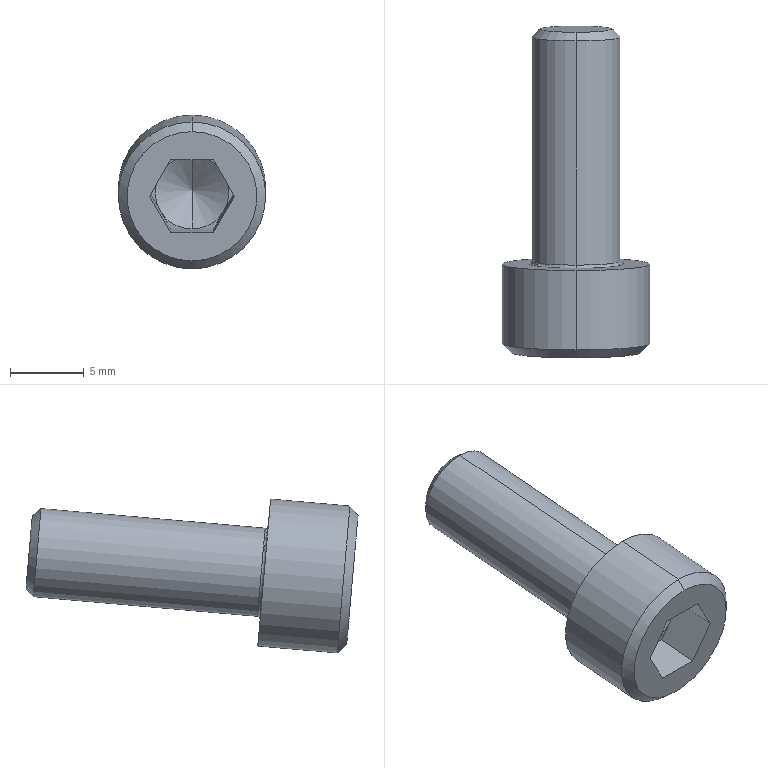Part | SolidWorks | features BaseBody 1 | 1 solid | 27 faces | box 10 x 22.514 x 10.433 mm | volume 841.351 mm3 | plane 15 | cone 6 | cylinder 4 | torus 2 | commonest cylinder face diameters 6 x2 10 x2
STEP:
#1=CARTESIAN_POINT('',(9.,-4.651,-13.958));
#2=VERTEX_POINT('',#1);
#3=CARTESIAN_POINT('',(5.8,-4.372,-17.146));
#4=VERTEX_POINT('',#3);
#5=CARTESIAN_POINT('',(9.,-4.651,-13.958));
#6=CARTESIAN_POINT('',(8.796,-4.651,-13.959));
#7=CARTESIAN_POINT('',(8.497,-4.649,-13.987));
#8=CARTESIAN_POINT('',(8.156,-4.642,-14.068));
#9=CARTESIAN_POINT('',(7.988,-4.637,-14.121));
#10=CARTESIAN_POINT('',(7.917,-4.635,-14.146));
#11=CARTESIAN_POINT('',(7.869,-4.633,-14.164));
#12=CARTESIAN_POINT('',(7.848,-4.632,-14.172));
#13=CARTESIAN_POINT('',(7.412,-4.617,-14.344));
#14=CARTESIAN_POINT('',(7.049,-4.597,-14.581));
#15=CARTESIAN_POINT('',(6.581,-4.556,-15.048));
#16=CARTESIAN_POINT('',(6.375,-4.534,-15.299));
#17=CARTESIAN_POINT('',(6.183,-4.505,-15.625));
#18=CARTESIAN_POINT('',(6.1,-4.49,-15.796));
#19=CARTESIAN_POINT('',(6.067,-4.484,-15.871));
#20=CARTESIAN_POINT('',(6.045,-4.479,-15.922));
#21=CARTESIAN_POINT('',(6.034,-4.477,-15.949));
#22=CARTESIAN_POINT('',(5.875,-4.442,-16.349));
#23=CARTESIAN_POINT('',(5.8,-4.408,-16.74));
#24=CARTESIAN_POINT('',(5.8,-4.372,-17.146));
#25=B_SPLINE_CURVE_WITH_KNOTS('',3,(#5,#6,#7,#8,#9,#10,#11,#12,#13,#14,#15,#16,#17,#18,#19,#20,#21,#22,#23,#24),.UNSPECIFIED.,.F.,.F.,(4,1,1,1,2,2,2,1,1,1,2,2,4),(0.,0.125,0.1875,0.2188,0.2344,0.25,0.5,0.625,0.6875,0.7187,0.7344,0.75,1.),.UNSPECIFIED.);
#26=EDGE_CURVE('',#2,#4,#25,.T.);
#27=ORIENTED_EDGE('',*,*,#26,.F.);
#28=CARTESIAN_POINT('',(9.,-4.434,-14.14));
#29=VERTEX_POINT('',#28);
#30=CARTESIAN_POINT('',(9.,-4.452,-13.941));
#31=DIRECTION('',(1.,0.,0.));
#32=DIRECTION('',(0.,1.,0.));
#33=AXIS2_PLACEMENT_3D('',#30,#31,#32);
#34=CIRCLE('',#33,0.2);
#35=EDGE_CURVE('',#2,#29,#34,.T.);
#36=ORIENTED_EDGE('',*,*,#35,.T.);
#37=CARTESIAN_POINT('',(9.,-3.912,-20.117));
#38=VERTEX_POINT('',#37);
#39=CARTESIAN_POINT('',(9.,-4.173,-17.129));
#40=DIRECTION('',(0.,0.9962,0.08716));
#41=DIRECTION('',(0.,-0.08716,0.9962));
#42=AXIS2_PLACEMENT_3D('',#39,#40,#41);
#43=CIRCLE('',#42,3.);
#44=EDGE_CURVE('',#38,#29,#43,.T.);
#45=ORIENTED_EDGE('',*,*,#44,.F.);
#46=CARTESIAN_POINT('',(9.,-4.093,-20.334));
#47=VERTEX_POINT('',#46);
#48=CARTESIAN_POINT('',(9.,-3.894,-20.317));
#49=DIRECTION('',(-1.,0.,0.));
#50=DIRECTION('',(0.,-1.,0.));
#51=AXIS2_PLACEMENT_3D('',#48,#49,#50);
#52=CIRCLE('',#51,0.2);
#53=EDGE_CURVE('',#47,#38,#52,.T.);
#54=ORIENTED_EDGE('',*,*,#53,.F.);
#55=CARTESIAN_POINT('',(5.8,-4.372,-17.146));
#56=CARTESIAN_POINT('',(5.8,-4.354,-17.349));
#57=CARTESIAN_POINT('',(5.828,-4.328,-17.648));
#58=CARTESIAN_POINT('',(5.91,-4.299,-17.987));
#59=CARTESIAN_POINT('',(5.963,-4.284,-18.154));
#60=CARTESIAN_POINT('',(5.989,-4.278,-18.225));
#61=CARTESIAN_POINT('',(6.006,-4.274,-18.273));
#62=CARTESIAN_POINT('',(6.015,-4.272,-18.294));
#63=CARTESIAN_POINT('',(6.187,-4.234,-18.729));
#64=CARTESIAN_POINT('',(6.425,-4.202,-19.089));
#65=CARTESIAN_POINT('',(6.893,-4.161,-19.556));
#66=CARTESIAN_POINT('',(7.146,-4.143,-19.761));
#67=CARTESIAN_POINT('',(7.473,-4.127,-19.952));
#68=CARTESIAN_POINT('',(7.645,-4.119,-20.035));
#69=CARTESIAN_POINT('',(7.72,-4.117,-20.068));
#70=CARTESIAN_POINT('',(7.771,-4.115,-20.09));
#71=CARTESIAN_POINT('',(7.798,-4.114,-20.101));
#72=CARTESIAN_POINT('',(8.2,-4.1,-20.259));
#73=CARTESIAN_POINT('',(8.593,-4.093,-20.334));
#74=CARTESIAN_POINT('',(9.,-4.093,-20.334));
#75=B_SPLINE_CURVE_WITH_KNOTS('',3,(#55,#56,#57,#58,#59,#60,#61,#62,#63,#64,#65,#66,#67,#68,#69,#70,#71,#72,#73,#74),.UNSPECIFIED.,.F.,.F.,(4,1,1,1,2,2,2,1,1,1,2,2,4),(0.,0.125,0.1875,0.2188,0.2344,0.25,0.5,0.625,0.6875,0.7188,0.7344,0.75,1.),.UNSPECIFIED.);
#76=EDGE_CURVE('',#4,#47,#75,.T.);
#77=ORIENTED_EDGE('',*,*,#76,.F.);
#78=EDGE_LOOP('',(#27,#36,#45,#54,#77));
#79=FACE_OUTER_BOUND('',#78,.T.);
#80=CARTESIAN_POINT('',(9.,-4.173,-17.129));
#81=DIRECTION('',(0.,-0.9962,-0.08716));
#82=DIRECTION('',(0.,0.08716,-0.9962));
#83=AXIS2_PLACEMENT_3D('',#80,#81,#82);
#84=TOROIDAL_SURFACE('',#83,3.2,0.2);
#85=ADVANCED_FACE('',(#79),#84,.F.);
#86=CARTESIAN_POINT('',(9.,-4.173,-17.129));
#87=DIRECTION('',(0.,0.9962,0.08716));
#88=DIRECTION('',(0.,-0.08716,0.9962));
#89=AXIS2_PLACEMENT_3D('',#86,#87,#88);
#90=CIRCLE('',#89,3.);
#91=EDGE_CURVE('',#29,#38,#90,.T.);
#92=ORIENTED_EDGE('',*,*,#91,.T.);
#93=CARTESIAN_POINT('',(9.,11.289,-18.788));
#94=VERTEX_POINT('',#93);
#95=CARTESIAN_POINT('',(9.,3.689,-19.453));
#96=DIRECTION('',(0.,0.9962,0.08716));
#97=VECTOR('',#96,1000.);
#98=LINE('',#95,#97);
#99=EDGE_CURVE('',#38,#94,#98,.T.);
#100=ORIENTED_EDGE('',*,*,#99,.T.);
#101=CARTESIAN_POINT('',(9.,10.766,-12.81));
#102=VERTEX_POINT('',#101);
#103=CARTESIAN_POINT('',(9.,11.027,-15.799));
#104=DIRECTION('',(0.,-0.9962,-0.08716));
#105=DIRECTION('',(0.,-0.08716,0.9962));
#106=AXIS2_PLACEMENT_3D('',#103,#104,#105);
#107=CIRCLE('',#106,3.);
#108=EDGE_CURVE('',#94,#102,#107,.T.);
#109=ORIENTED_EDGE('',*,*,#108,.T.);
#110=CARTESIAN_POINT('',(9.,3.166,-13.475));
#111=DIRECTION('',(0.,0.9962,0.08716));
#112=VECTOR('',#111,1000.);
#113=LINE('',#110,#112);
#114=EDGE_CURVE('',#29,#102,#113,.T.);
#115=ORIENTED_EDGE('',*,*,#114,.F.);
#116=EDGE_LOOP('',(#92,#100,#109,#115));
#117=FACE_OUTER_BOUND('',#116,.T.);
#118=CARTESIAN_POINT('',(9.,3.427,-16.464));
#119=DIRECTION('',(0.,0.9962,0.08716));
#120=DIRECTION('',(0.,-0.08716,0.9962));
#121=AXIS2_PLACEMENT_3D('',#118,#119,#120);
#122=CYLINDRICAL_SURFACE('',#121,3.);
#123=ADVANCED_FACE('',(#117),#122,.T.);
#124=CARTESIAN_POINT('',(9.,11.781,-18.201));
#125=VERTEX_POINT('',#124);
#126=CARTESIAN_POINT('',(9.,11.353,-13.303));
#127=VERTEX_POINT('',#126);
#128=CARTESIAN_POINT('',(9.,11.567,-15.752));
#129=DIRECTION('',(0.,-0.9962,-0.08716));
#130=DIRECTION('',(0.,0.08716,-0.9962));
#131=AXIS2_PLACEMENT_3D('',#128,#129,#130);
#132=CIRCLE('',#131,2.458);
#133=EDGE_CURVE('',#125,#127,#132,.T.);
#134=ORIENTED_EDGE('',*,*,#133,.T.);
#135=CARTESIAN_POINT('',(9.,10.766,-12.81));
#136=DIRECTION('',(0.,-0.766,0.6428));
#137=VECTOR('',#136,1000.);
#138=LINE('',#135,#137);
#139=EDGE_CURVE('',#127,#102,#138,.T.);
#140=ORIENTED_EDGE('',*,*,#139,.T.);
#141=ORIENTED_EDGE('',*,*,#108,.F.);
#142=CARTESIAN_POINT('',(9.,11.289,-18.788));
#143=DIRECTION('',(0.,-0.6428,-0.766));
#144=VECTOR('',#143,1000.);
#145=LINE('',#142,#144);
#146=EDGE_CURVE('',#125,#94,#145,.T.);
#147=ORIENTED_EDGE('',*,*,#146,.F.);
#148=EDGE_LOOP('',(#134,#140,#141,#147));
#149=FACE_OUTER_BOUND('',#148,.T.);
#150=CARTESIAN_POINT('',(9.,11.027,-15.799));
#151=DIRECTION('',(0.,-0.9962,-0.08716));
#152=DIRECTION('',(0.,0.08716,-0.9962));
#153=AXIS2_PLACEMENT_3D('',#150,#151,#152);
#154=CONICAL_SURFACE('',#153,3.,0.7854);
#155=ADVANCED_FACE('',(#149),#154,.T.);
#156=CARTESIAN_POINT('',(9.,-10.187,-12.636));
#157=VERTEX_POINT('',#156);
#158=CARTESIAN_POINT('',(9.,-9.316,-22.598));
#159=VERTEX_POINT('',#158);
#160=CARTESIAN_POINT('',(9.,-9.752,-17.617));
#161=DIRECTION('',(0.,0.9962,0.08716));
#162=DIRECTION('',(0.,-0.08716,0.9962));
#163=AXIS2_PLACEMENT_3D('',#160,#161,#162);
#164=CIRCLE('',#163,5.);
#165=EDGE_CURVE('',#157,#159,#164,.T.);
#166=ORIENTED_EDGE('',*,*,#165,.T.);
#167=CARTESIAN_POINT('',(9.,-3.936,-22.127));
#168=VERTEX_POINT('',#167);
#169=CARTESIAN_POINT('',(9.,-6.626,-22.363));
#170=DIRECTION('',(0.,0.9962,0.08716));
#171=VECTOR('',#170,1000.);
#172=LINE('',#169,#171);
#173=EDGE_CURVE('',#159,#168,#172,.T.);
#174=ORIENTED_EDGE('',*,*,#173,.T.);
#175=CARTESIAN_POINT('',(9.,-4.808,-12.165));
#176=VERTEX_POINT('',#175);
#177=CARTESIAN_POINT('',(9.,-4.372,-17.146));
#178=DIRECTION('',(0.,0.9962,0.08716));
#179=DIRECTION('',(0.,-0.08716,0.9962));
#180=AXIS2_PLACEMENT_3D('',#177,#178,#179);
#181=CIRCLE('',#180,5.);
#182=EDGE_CURVE('',#176,#168,#181,.T.);
#183=ORIENTED_EDGE('',*,*,#182,.F.);
#184=CARTESIAN_POINT('',(9.,-7.498,-12.401));
#185=DIRECTION('',(0.,0.9962,0.08716));
#186=VECTOR('',#185,1000.);
#187=LINE('',#184,#186);
#188=EDGE_CURVE('',#157,#176,#187,.T.);
#189=ORIENTED_EDGE('',*,*,#188,.F.);
#190=EDGE_LOOP('',(#166,#174,#183,#189));
#191=FACE_OUTER_BOUND('',#190,.T.);
#192=CARTESIAN_POINT('',(9.,-7.062,-17.382));
#193=DIRECTION('',(0.,0.9962,0.08716));
#194=DIRECTION('',(0.,-0.08716,0.9962));
#195=AXIS2_PLACEMENT_3D('',#192,#193,#194);
#196=CYLINDRICAL_SURFACE('',#195,5.);
#197=ADVANCED_FACE('',(#191),#196,.T.);
#198=CARTESIAN_POINT('',(9.,-10.733,-13.286));
#199=VERTEX_POINT('',#198);
#200=CARTESIAN_POINT('',(9.,-9.966,-22.053));
#201=VERTEX_POINT('',#200);
#202=CARTESIAN_POINT('',(9.,-10.349,-17.669));
#203=DIRECTION('',(0.,0.9962,0.08716));
#204=DIRECTION('',(0.,-0.08716,0.9962));
#205=AXIS2_PLACEMENT_3D('',#202,#203,#204);
#206=CIRCLE('',#205,4.4);
#207=EDGE_CURVE('',#199,#201,#206,.T.);
#208=ORIENTED_EDGE('',*,*,#207,.T.);
#209=CARTESIAN_POINT('',(9.,-9.316,-22.598));
#210=DIRECTION('',(0.,0.766,-0.6428));
#211=VECTOR('',#210,1000.);
#212=LINE('',#209,#211);
#213=EDGE_CURVE('',#201,#159,#212,.T.);
#214=ORIENTED_EDGE('',*,*,#213,.T.);
#215=ORIENTED_EDGE('',*,*,#165,.F.);
#216=CARTESIAN_POINT('',(9.,-10.187,-12.636));
#217=DIRECTION('',(0.,0.6428,0.766));
#218=VECTOR('',#217,1000.);
#219=LINE('',#216,#218);
#220=EDGE_CURVE('',#199,#157,#219,.T.);
#221=ORIENTED_EDGE('',*,*,#220,.F.);
#222=EDGE_LOOP('',(#208,#214,#215,#221));
#223=FACE_OUTER_BOUND('',#222,.T.);
#224=CARTESIAN_POINT('',(9.,-9.752,-17.617));
#225=DIRECTION('',(0.,0.9962,0.08716));
#226=DIRECTION('',(0.,-0.08716,0.9962));
#227=AXIS2_PLACEMENT_3D('',#224,#225,#226);
#228=CONICAL_SURFACE('',#227,5.,0.7854);
#229=ADVANCED_FACE('',(#223),#228,.T.);
#230=CARTESIAN_POINT('',(9.,-5.923,-17.282));
#231=VERTEX_POINT('',#230);
#232=CARTESIAN_POINT('',(9.,-7.143,-19.898));
#233=VERTEX_POINT('',#232);
#234=CARTESIAN_POINT('',(9.,-7.143,-19.898));
#235=DIRECTION('',(0.,-0.4226,-0.9063));
#236=VECTOR('',#235,1000.);
#237=LINE('',#234,#236);
#238=EDGE_CURVE('',#231,#233,#237,.T.);
#239=ORIENTED_EDGE('',*,*,#238,.F.);
#240=CARTESIAN_POINT('',(9.,-7.579,-14.917));
#241=VERTEX_POINT('',#240);
#242=CARTESIAN_POINT('',(9.,-7.579,-14.917));
#243=DIRECTION('',(0.,-0.5736,0.8192));
#244=VECTOR('',#243,1000.);
#245=LINE('',#242,#244);
#246=EDGE_CURVE('',#231,#241,#245,.T.);
#247=ORIENTED_EDGE('',*,*,#246,.T.);
#248=CARTESIAN_POINT('',(6.835,-7.47,-16.163));
#249=VERTEX_POINT('',#248);
#250=CARTESIAN_POINT('',(9.,-7.361,-17.408));
#251=DIRECTION('',(0.,-0.9962,-0.08716));
#252=DIRECTION('',(0.,0.08716,-0.9962));
#253=AXIS2_PLACEMENT_3D('',#250,#251,#252);
#254=CIRCLE('',#253,2.5);
#255=EDGE_CURVE('',#241,#249,#254,.T.);
#256=ORIENTED_EDGE('',*,*,#255,.T.);
#257=CARTESIAN_POINT('',(6.835,-7.252,-18.653));
#258=VERTEX_POINT('',#257);
#259=CARTESIAN_POINT('',(9.,-7.361,-17.408));
#260=DIRECTION('',(0.,0.9962,0.08716));
#261=DIRECTION('',(0.,0.08716,-0.9962));
#262=AXIS2_PLACEMENT_3D('',#259,#260,#261);
#263=CIRCLE('',#262,2.5);
#264=EDGE_CURVE('',#258,#249,#263,.T.);
#265=ORIENTED_EDGE('',*,*,#264,.F.);
#266=CARTESIAN_POINT('',(9.,-7.361,-17.408));
#267=DIRECTION('',(0.,0.9962,0.08716));
#268=DIRECTION('',(0.,0.08716,-0.9962));
#269=AXIS2_PLACEMENT_3D('',#266,#267,#268);
#270=CIRCLE('',#269,2.5);
#271=EDGE_CURVE('',#233,#258,#270,.T.);
#272=ORIENTED_EDGE('',*,*,#271,.F.);
#273=EDGE_LOOP('',(#239,#247,#256,#265,#272));
#274=FACE_OUTER_BOUND('',#273,.T.);
#275=CARTESIAN_POINT('',(9.,-7.361,-17.408));
#276=DIRECTION('',(0.,-0.9962,-0.08716));
#277=DIRECTION('',(0.,0.08716,-0.9962));
#278=AXIS2_PLACEMENT_3D('',#275,#276,#277);
#279=CONICAL_SURFACE('',#278,2.5,1.047);
#280=ADVANCED_FACE('',(#274),#279,.F.);
#281=CARTESIAN_POINT('',(10.443,-7.143,-19.898));
#282=VERTEX_POINT('',#281);
#283=CARTESIAN_POINT('',(9.,-7.143,-19.898));
#284=DIRECTION('',(-1.,0.,0.));
#285=VECTOR('',#284,1000.);
#286=LINE('',#283,#285);
#287=EDGE_CURVE('',#282,#233,#286,.T.);
#288=ORIENTED_EDGE('',*,*,#287,.F.);
#289=CARTESIAN_POINT('',(11.165,-7.252,-18.653));
#290=VERTEX_POINT('',#289);
#291=CARTESIAN_POINT('',(11.165,-7.252,-18.653));
#292=DIRECTION('',(-0.5,0.07548,-0.8627));
#293=VECTOR('',#292,1000.);
#294=LINE('',#291,#293);
#295=EDGE_CURVE('',#290,#282,#294,.T.);
#296=ORIENTED_EDGE('',*,*,#295,.F.);
#297=CARTESIAN_POINT('',(9.,-7.361,-17.408));
#298=DIRECTION('',(0.,0.9962,0.08716));
#299=DIRECTION('',(0.,0.08716,-0.9962));
#300=AXIS2_PLACEMENT_3D('',#297,#298,#299);
#301=CIRCLE('',#300,2.5);
#302=EDGE_CURVE('',#290,#233,#301,.T.);
#303=ORIENTED_EDGE('',*,*,#302,.T.);
#304=EDGE_LOOP('',(#288,#296,#303));
#305=FACE_OUTER_BOUND('',#304,.T.);
#306=CARTESIAN_POINT('',(9.,-7.361,-17.408));
#307=DIRECTION('',(0.,0.9962,0.08716));
#308=DIRECTION('',(1.,0.,0.));
#309=AXIS2_PLACEMENT_3D('',#306,#307,#308);
#310=PLANE('',#309);
#311=ADVANCED_FACE('',(#305),#310,.F.);
#312=CARTESIAN_POINT('',(7.557,-7.143,-19.898));
#313=VERTEX_POINT('',#312);
#314=CARTESIAN_POINT('',(7.557,-7.143,-19.898));
#315=DIRECTION('',(-0.5,-0.07548,0.8627));
#316=VECTOR('',#315,1000.);
#317=LINE('',#314,#316);
#318=EDGE_CURVE('',#313,#258,#317,.T.);
#319=ORIENTED_EDGE('',*,*,#318,.F.);
#320=CARTESIAN_POINT('',(9.,-7.143,-19.898));
#321=DIRECTION('',(-1.,0.,0.));
#322=VECTOR('',#321,1000.);
#323=LINE('',#320,#322);
#324=EDGE_CURVE('',#233,#313,#323,.T.);
#325=ORIENTED_EDGE('',*,*,#324,.F.);
#326=ORIENTED_EDGE('',*,*,#271,.T.);
#327=EDGE_LOOP('',(#319,#325,#326));
#328=FACE_OUTER_BOUND('',#327,.T.);
#329=CARTESIAN_POINT('',(9.,-7.361,-17.408));
#330=DIRECTION('',(0.,0.9962,0.08716));
#331=DIRECTION('',(1.,0.,0.));
#332=AXIS2_PLACEMENT_3D('',#329,#330,#331);
#333=PLANE('',#332);
#334=ADVANCED_FACE('',(#328),#333,.F.);
#335=CARTESIAN_POINT('',(10.443,-7.579,-14.917));
#336=VERTEX_POINT('',#335);
#337=CARTESIAN_POINT('',(11.165,-7.47,-16.163));
#338=VERTEX_POINT('',#337);
#339=CARTESIAN_POINT('',(10.443,-7.579,-14.917));
#340=DIRECTION('',(0.5,0.07548,-0.8627));
#341=VECTOR('',#340,1000.);
#342=LINE('',#339,#341);
#343=EDGE_CURVE('',#336,#338,#342,.T.);
#344=ORIENTED_EDGE('',*,*,#343,.F.);
#345=CARTESIAN_POINT('',(9.,-7.579,-14.917));
#346=DIRECTION('',(1.,0.,0.));
#347=VECTOR('',#346,1000.);
#348=LINE('',#345,#347);
#349=EDGE_CURVE('',#241,#336,#348,.T.);
#350=ORIENTED_EDGE('',*,*,#349,.F.);
#351=CARTESIAN_POINT('',(9.,-7.361,-17.408));
#352=DIRECTION('',(0.,0.9962,0.08716));
#353=DIRECTION('',(0.,0.08716,-0.9962));
#354=AXIS2_PLACEMENT_3D('',#351,#352,#353);
#355=CIRCLE('',#354,2.5);
#356=EDGE_CURVE('',#241,#338,#355,.T.);
#357=ORIENTED_EDGE('',*,*,#356,.T.);
#358=EDGE_LOOP('',(#344,#350,#357));
#359=FACE_OUTER_BOUND('',#358,.T.);
#360=CARTESIAN_POINT('',(9.,-7.361,-17.408));
#361=DIRECTION('',(0.,0.9962,0.08716));
#362=DIRECTION('',(1.,0.,0.));
#363=AXIS2_PLACEMENT_3D('',#360,#361,#362);
#364=PLANE('',#363);
#365=ADVANCED_FACE('',(#359),#364,.F.);
#366=CARTESIAN_POINT('',(7.557,-7.579,-14.917));
#367=VERTEX_POINT('',#366);
#368=CARTESIAN_POINT('',(10.443,-7.579,-14.917));
#369=DIRECTION('',(-1.,0.,0.));
#370=VECTOR('',#369,1000.);
#371=LINE('',#368,#370);
#372=EDGE_CURVE('',#241,#367,#371,.T.);
#373=ORIENTED_EDGE('',*,*,#372,.T.);
#374=CARTESIAN_POINT('',(7.557,-7.579,-14.917));
#375=DIRECTION('',(-0.5,0.07548,-0.8627));
#376=VECTOR('',#375,1000.);
#377=LINE('',#374,#376);
#378=EDGE_CURVE('',#367,#249,#377,.T.);
#379=ORIENTED_EDGE('',*,*,#378,.T.);
#380=ORIENTED_EDGE('',*,*,#255,.F.);
#381=EDGE_LOOP('',(#373,#379,#380));
#382=FACE_OUTER_BOUND('',#381,.T.);
#383=CARTESIAN_POINT('',(9.,-7.361,-17.408));
#384=DIRECTION('',(0.,0.9962,0.08716));
#385=DIRECTION('',(1.,0.,0.));
#386=AXIS2_PLACEMENT_3D('',#383,#384,#385);
#387=PLANE('',#386);
#388=ADVANCED_FACE('',(#382),#387,.F.);
#389=CARTESIAN_POINT('',(9.,-7.361,-17.408));
#390=DIRECTION('',(0.,0.9962,0.08716));
#391=DIRECTION('',(0.,0.08716,-0.9962));
#392=AXIS2_PLACEMENT_3D('',#389,#390,#391);
#393=CIRCLE('',#392,2.5);
#394=EDGE_CURVE('',#338,#290,#393,.T.);
#395=ORIENTED_EDGE('',*,*,#394,.T.);
#396=CARTESIAN_POINT('',(11.887,-7.361,-17.408));
#397=VERTEX_POINT('',#396);
#398=CARTESIAN_POINT('',(11.165,-7.252,-18.653));
#399=DIRECTION('',(0.5,-0.07548,0.8627));
#400=VECTOR('',#399,1000.);
#401=LINE('',#398,#400);
#402=EDGE_CURVE('',#290,#397,#401,.T.);
#403=ORIENTED_EDGE('',*,*,#402,.T.);
#404=CARTESIAN_POINT('',(11.887,-7.361,-17.408));
#405=DIRECTION('',(-0.5,-0.07548,0.8627));
#406=VECTOR('',#405,1000.);
#407=LINE('',#404,#406);
#408=EDGE_CURVE('',#397,#338,#407,.T.);
#409=ORIENTED_EDGE('',*,*,#408,.T.);
#410=EDGE_LOOP('',(#395,#403,#409));
#411=FACE_OUTER_BOUND('',#410,.T.);
#412=CARTESIAN_POINT('',(9.,-7.361,-17.408));
#413=DIRECTION('',(0.,0.9962,0.08716));
#414=DIRECTION('',(1.,0.,0.));
#415=AXIS2_PLACEMENT_3D('',#412,#413,#414);
#416=PLANE('',#415);
#417=ADVANCED_FACE('',(#411),#416,.F.);
#418=ORIENTED_EDGE('',*,*,#264,.T.);
#419=CARTESIAN_POINT('',(6.113,-7.361,-17.408));
#420=VERTEX_POINT('',#419);
#421=CARTESIAN_POINT('',(6.835,-7.47,-16.163));
#422=DIRECTION('',(-0.5,0.07548,-0.8627));
#423=VECTOR('',#422,1000.);
#424=LINE('',#421,#423);
#425=EDGE_CURVE('',#249,#420,#424,.T.);
#426=ORIENTED_EDGE('',*,*,#425,.T.);
#427=CARTESIAN_POINT('',(6.113,-7.361,-17.408));
#428=DIRECTION('',(0.5,0.07548,-0.8627));
#429=VECTOR('',#428,1000.);
#430=LINE('',#427,#429);
#431=EDGE_CURVE('',#420,#258,#430,.T.);
#432=ORIENTED_EDGE('',*,*,#431,.T.);
#433=EDGE_LOOP('',(#418,#426,#432));
#434=FACE_OUTER_BOUND('',#433,.T.);
#435=CARTESIAN_POINT('',(9.,-7.361,-17.408));
#436=DIRECTION('',(0.,0.9962,0.08716));
#437=DIRECTION('',(1.,0.,0.));
#438=AXIS2_PLACEMENT_3D('',#435,#436,#437);
#439=PLANE('',#438);
#440=ADVANCED_FACE('',(#434),#439,.F.);
#441=CARTESIAN_POINT('',(7.557,-10.567,-15.179));
#442=VERTEX_POINT('',#441);
#443=CARTESIAN_POINT('',(7.557,-10.567,-15.179));
#444=DIRECTION('',(0.,-0.9962,-0.08716));
#445=VECTOR('',#444,1000.);
#446=LINE('',#443,#445);
#447=EDGE_CURVE('',#367,#442,#446,.T.);
#448=ORIENTED_EDGE('',*,*,#447,.T.);
#449=CARTESIAN_POINT('',(6.113,-10.349,-17.669));
#450=VERTEX_POINT('',#449);
#451=CARTESIAN_POINT('',(6.113,-10.349,-17.669));
#452=DIRECTION('',(0.5,-0.07548,0.8627));
#453=VECTOR('',#452,1000.);
#454=LINE('',#451,#453);
#455=EDGE_CURVE('',#450,#442,#454,.T.);
#456=ORIENTED_EDGE('',*,*,#455,.F.);
#457=CARTESIAN_POINT('',(6.113,-10.349,-17.669));
#458=DIRECTION('',(0.,0.9962,0.08716));
#459=VECTOR('',#458,1000.);
#460=LINE('',#457,#459);
#461=EDGE_CURVE('',#450,#420,#460,.T.);
#462=ORIENTED_EDGE('',*,*,#461,.T.);
#463=ORIENTED_EDGE('',*,*,#425,.F.);
#464=ORIENTED_EDGE('',*,*,#378,.F.);
#465=EDGE_LOOP('',(#448,#456,#462,#463,#464));
#466=FACE_OUTER_BOUND('',#465,.T.);
#467=CARTESIAN_POINT('',(7.557,-10.567,-15.179));
#468=DIRECTION('',(-0.866,-0.04358,0.4981));
#469=DIRECTION('',(-0.05026,0.9987,0.));
#470=AXIS2_PLACEMENT_3D('',#467,#468,#469);
#471=PLANE('',#470);
#472=ADVANCED_FACE('',(#466),#471,.F.);
#473=CARTESIAN_POINT('',(10.443,-10.567,-15.179));
#474=VERTEX_POINT('',#473);
#475=CARTESIAN_POINT('',(10.443,-7.579,-14.917));
#476=DIRECTION('',(0.,-0.9962,-0.08716));
#477=VECTOR('',#476,1000.);
#478=LINE('',#475,#477);
#479=EDGE_CURVE('',#336,#474,#478,.T.);
#480=ORIENTED_EDGE('',*,*,#479,.T.);
#481=CARTESIAN_POINT('',(6.8,-10.567,-15.179));
#482=DIRECTION('',(1.,0.,0.));
#483=VECTOR('',#482,1000.);
#484=LINE('',#481,#483);
#485=EDGE_CURVE('',#442,#474,#484,.T.);
#486=ORIENTED_EDGE('',*,*,#485,.F.);
#487=ORIENTED_EDGE('',*,*,#447,.F.);
#488=ORIENTED_EDGE('',*,*,#372,.F.);
#489=ORIENTED_EDGE('',*,*,#349,.T.);
#490=EDGE_LOOP('',(#480,#486,#487,#488,#489));
#491=FACE_OUTER_BOUND('',#490,.T.);
#492=CARTESIAN_POINT('',(10.443,-10.567,-15.179));
#493=DIRECTION('',(0.,-0.08716,0.9962));
#494=DIRECTION('',(-1.,0.,0.));
#495=AXIS2_PLACEMENT_3D('',#492,#493,#494);
#496=PLANE('',#495);
#497=ADVANCED_FACE('',(#491),#496,.F.);
#498=CARTESIAN_POINT('',(11.887,-10.349,-17.669));
#499=VERTEX_POINT('',#498);
#500=CARTESIAN_POINT('',(11.887,-7.361,-17.408));
#501=DIRECTION('',(0.,-0.9962,-0.08716));
#502=VECTOR('',#501,1000.);
#503=LINE('',#500,#502);
#504=EDGE_CURVE('',#397,#499,#503,.T.);
#505=ORIENTED_EDGE('',*,*,#504,.T.);
#506=CARTESIAN_POINT('',(10.443,-10.567,-15.179));
#507=DIRECTION('',(0.5,0.07548,-0.8627));
#508=VECTOR('',#507,1000.);
#509=LINE('',#506,#508);
#510=EDGE_CURVE('',#474,#499,#509,.T.);
#511=ORIENTED_EDGE('',*,*,#510,.F.);
#512=ORIENTED_EDGE('',*,*,#479,.F.);
#513=ORIENTED_EDGE('',*,*,#343,.T.);
#514=ORIENTED_EDGE('',*,*,#408,.F.);
#515=EDGE_LOOP('',(#505,#511,#512,#513,#514));
#516=FACE_OUTER_BOUND('',#515,.T.);
#517=CARTESIAN_POINT('',(11.887,-10.349,-17.669));
#518=DIRECTION('',(0.866,-0.04358,0.4981));
#519=DIRECTION('',(0.,-0.9962,-0.08716));
#520=AXIS2_PLACEMENT_3D('',#517,#518,#519);
#521=PLANE('',#520);
#522=ADVANCED_FACE('',(#516),#521,.F.);
#523=CARTESIAN_POINT('',(10.443,-10.132,-20.16));
#524=VERTEX_POINT('',#523);
#525=CARTESIAN_POINT('',(10.443,-10.132,-20.16));
#526=DIRECTION('',(0.,-0.9962,-0.08716));
#527=VECTOR('',#526,1000.);
#528=LINE('',#525,#527);
#529=EDGE_CURVE('',#282,#524,#528,.T.);
#530=ORIENTED_EDGE('',*,*,#529,.T.);
#531=CARTESIAN_POINT('',(11.887,-10.349,-17.669));
#532=DIRECTION('',(-0.5,0.07548,-0.8627));
#533=VECTOR('',#532,1000.);
#534=LINE('',#531,#533);
#535=EDGE_CURVE('',#499,#524,#534,.T.);
#536=ORIENTED_EDGE('',*,*,#535,.F.);
#537=ORIENTED_EDGE('',*,*,#504,.F.);
#538=ORIENTED_EDGE('',*,*,#402,.F.);
#539=ORIENTED_EDGE('',*,*,#295,.T.);
#540=EDGE_LOOP('',(#530,#536,#537,#538,#539));
#541=FACE_OUTER_BOUND('',#540,.T.);
#542=CARTESIAN_POINT('',(10.443,-10.132,-20.16));
#543=DIRECTION('',(0.866,0.04358,-0.4981));
#544=DIRECTION('',(0.,-0.9962,-0.08716));
#545=AXIS2_PLACEMENT_3D('',#542,#543,#544);
#546=PLANE('',#545);
#547=ADVANCED_FACE('',(#541),#546,.F.);
#548=CARTESIAN_POINT('',(7.557,-10.132,-20.16));
#549=VERTEX_POINT('',#548);
#550=CARTESIAN_POINT('',(7.557,-7.143,-19.898));
#551=DIRECTION('',(0.,-0.9962,-0.08716));
#552=VECTOR('',#551,1000.);
#553=LINE('',#550,#552);
#554=EDGE_CURVE('',#313,#549,#553,.T.);
#555=ORIENTED_EDGE('',*,*,#554,.T.);
#556=CARTESIAN_POINT('',(6.8,-10.132,-20.16));
#557=DIRECTION('',(-1.,0.,0.));
#558=VECTOR('',#557,1000.);
#559=LINE('',#556,#558);
#560=EDGE_CURVE('',#524,#549,#559,.T.);
#561=ORIENTED_EDGE('',*,*,#560,.F.);
#562=ORIENTED_EDGE('',*,*,#529,.F.);
#563=ORIENTED_EDGE('',*,*,#287,.T.);
#564=ORIENTED_EDGE('',*,*,#324,.T.);
#565=EDGE_LOOP('',(#555,#561,#562,#563,#564));
#566=FACE_OUTER_BOUND('',#565,.T.);
#567=CARTESIAN_POINT('',(7.557,-10.132,-20.16));
#568=DIRECTION('',(0.,0.08716,-0.9962));
#569=DIRECTION('',(-1.,0.,0.));
#570=AXIS2_PLACEMENT_3D('',#567,#568,#569);
#571=PLANE('',#570);
#572=ADVANCED_FACE('',(#566),#571,.F.);
#573=ORIENTED_EDGE('',*,*,#461,.F.);
#574=CARTESIAN_POINT('',(7.557,-10.132,-20.16));
#575=DIRECTION('',(-0.5,-0.07548,0.8627));
#576=VECTOR('',#575,1000.);
#577=LINE('',#574,#576);
#578=EDGE_CURVE('',#549,#450,#577,.T.);
#579=ORIENTED_EDGE('',*,*,#578,.F.);
#580=ORIENTED_EDGE('',*,*,#554,.F.);
#581=ORIENTED_EDGE('',*,*,#318,.T.);
#582=ORIENTED_EDGE('',*,*,#431,.F.);
#583=EDGE_LOOP('',(#573,#579,#580,#581,#582));
#584=FACE_OUTER_BOUND('',#583,.T.);
#585=CARTESIAN_POINT('',(6.113,-10.349,-17.669));
#586=DIRECTION('',(-0.866,0.04358,-0.4981));
#587=DIRECTION('',(-0.4986,0.,0.8668));
#588=AXIS2_PLACEMENT_3D('',#585,#586,#587);
#589=PLANE('',#588);
#590=ADVANCED_FACE('',(#584),#589,.F.);
#591=ORIENTED_EDGE('',*,*,#560,.T.);
#592=ORIENTED_EDGE('',*,*,#578,.T.);
#593=ORIENTED_EDGE('',*,*,#455,.T.);
#594=ORIENTED_EDGE('',*,*,#485,.T.);
#595=ORIENTED_EDGE('',*,*,#510,.T.);
#596=ORIENTED_EDGE('',*,*,#535,.T.);
#597=EDGE_LOOP('',(#591,#592,#593,#594,#595,#596));
#598=FACE_BOUND('',#597,.T.);
#599=ORIENTED_EDGE('',*,*,#207,.F.);
#600=CARTESIAN_POINT('',(9.,-10.349,-17.669));
#601=DIRECTION('',(0.,0.9962,0.08716));
#602=DIRECTION('',(0.,-0.08716,0.9962));
#603=AXIS2_PLACEMENT_3D('',#600,#601,#602);
#604=CIRCLE('',#603,4.4);
#605=EDGE_CURVE('',#201,#199,#604,.T.);
#606=ORIENTED_EDGE('',*,*,#605,.F.);
#607=EDGE_LOOP('',(#599,#606));
#608=FACE_OUTER_BOUND('',#607,.T.);
#609=CARTESIAN_POINT('',(6.8,-10.349,-17.669));
#610=DIRECTION('',(0.,-0.9962,-0.08716));
#611=DIRECTION('',(0.,0.08716,-0.9962));
#612=AXIS2_PLACEMENT_3D('',#609,#610,#611);
#613=PLANE('',#612);
#614=ADVANCED_FACE('',(#598,#608),#613,.T.);
#615=ORIENTED_EDGE('',*,*,#133,.F.);
#616=CARTESIAN_POINT('',(9.,11.567,-15.752));
#617=DIRECTION('',(0.,-0.9962,-0.08716));
#618=DIRECTION('',(0.,0.08716,-0.9962));
#619=AXIS2_PLACEMENT_3D('',#616,#617,#618);
#620=CIRCLE('',#619,2.458);
#621=EDGE_CURVE('',#127,#125,#620,.T.);
#622=ORIENTED_EDGE('',*,*,#621,.F.);
#623=EDGE_LOOP('',(#615,#622));
#624=FACE_OUTER_BOUND('',#623,.T.);
#625=CARTESIAN_POINT('',(7.771,11.567,-15.752));
#626=DIRECTION('',(0.,0.9962,0.08716));
#627=DIRECTION('',(1.,0.,0.));
#628=AXIS2_PLACEMENT_3D('',#625,#626,#627);
#629=PLANE('',#628);
#630=ADVANCED_FACE('',(#624),#629,.T.);
#631=CARTESIAN_POINT('',(9.,-4.093,-20.334));
#632=CARTESIAN_POINT('',(9.204,-4.093,-20.334));
#633=CARTESIAN_POINT('',(9.503,-4.096,-20.306));
#634=CARTESIAN_POINT('',(9.844,-4.103,-20.224));
#635=CARTESIAN_POINT('',(10.012,-4.108,-20.171));
#636=CARTESIAN_POINT('',(10.083,-4.11,-20.146));
#637=CARTESIAN_POINT('',(10.131,-4.111,-20.129));
#638=CARTESIAN_POINT('',(10.152,-4.112,-20.12));
#639=CARTESIAN_POINT('',(10.588,-4.127,-19.948));
#640=CARTESIAN_POINT('',(10.951,-4.148,-19.711));
#641=CARTESIAN_POINT('',(11.419,-4.189,-19.245));
#642=CARTESIAN_POINT('',(11.625,-4.211,-18.993));
#643=CARTESIAN_POINT('',(11.817,-4.239,-18.667));
#644=CARTESIAN_POINT('',(11.9,-4.254,-18.496));
#645=CARTESIAN_POINT('',(11.933,-4.261,-18.421));
#646=CARTESIAN_POINT('',(11.955,-4.265,-18.371));
#647=CARTESIAN_POINT('',(11.966,-4.268,-18.343));
#648=CARTESIAN_POINT('',(12.125,-4.303,-17.943));
#649=CARTESIAN_POINT('',(12.2,-4.337,-17.551));
#650=CARTESIAN_POINT('',(12.2,-4.39,-16.944));
#651=CARTESIAN_POINT('',(12.172,-4.416,-16.645));
#652=CARTESIAN_POINT('',(12.09,-4.446,-16.306));
#653=CARTESIAN_POINT('',(12.037,-4.46,-16.139));
#654=CARTESIAN_POINT('',(12.011,-4.467,-16.067));
#655=CARTESIAN_POINT('',(11.994,-4.471,-16.02));
#656=CARTESIAN_POINT('',(11.985,-4.473,-15.998));
#657=CARTESIAN_POINT('',(11.813,-4.511,-15.564));
#658=CARTESIAN_POINT('',(11.575,-4.542,-15.203));
#659=CARTESIAN_POINT('',(11.107,-4.583,-14.737));
#660=CARTESIAN_POINT('',(10.854,-4.601,-14.531));
#661=CARTESIAN_POINT('',(10.527,-4.618,-14.341));
#662=CARTESIAN_POINT('',(10.355,-4.625,-14.257));
#663=CARTESIAN_POINT('',(10.28,-4.628,-14.224));
#664=CARTESIAN_POINT('',(10.229,-4.63,-14.203));
#665=CARTESIAN_POINT('',(10.202,-4.631,-14.192));
#666=CARTESIAN_POINT('',(9.8,-4.645,-14.033));
#667=CARTESIAN_POINT('',(9.407,-4.651,-13.959));
#668=CARTESIAN_POINT('',(9.,-4.651,-13.958));
#669=B_SPLINE_CURVE_WITH_KNOTS('',3,(#631,#632,#633,#634,#635,#636,#637,#638,#639,#640,#641,#642,#643,#644,#645,#646,#647,#648,#649,#650,#651,#652,#653,#654,#655,#656,#657,#658,#659,#660,#661,#662,#663,#664,#665,#666,#667,#668),.UNSPECIFIED.,.F.,.F.,(4,1,1,1,2,2,2,1,1,1,2,2,2,1,1,1,2,2,2,1,1,1,2,2,4),(0.,0.0625,0.09375,0.1094,0.1172,0.125,0.25,0.3125,0.3437,0.3594,0.3672,0.375,0.5,0.5625,0.5937,0.6094,0.6172,0.625,0.75,0.8125,0.8437,0.8594,0.8672,0.875,1.),.UNSPECIFIED.);
#670=EDGE_CURVE('',#47,#2,#669,.T.);
#671=ORIENTED_EDGE('',*,*,#670,.T.);
#672=ORIENTED_EDGE('',*,*,#26,.T.);
#673=ORIENTED_EDGE('',*,*,#76,.T.);
#674=EDGE_LOOP('',(#671,#672,#673));
#675=FACE_BOUND('',#674,.T.);
#676=ORIENTED_EDGE('',*,*,#182,.T.);
#677=CARTESIAN_POINT('',(9.,-4.372,-17.146));
#678=DIRECTION('',(0.,0.9962,0.08716));
#679=DIRECTION('',(0.,-0.08716,0.9962));
#680=AXIS2_PLACEMENT_3D('',#677,#678,#679);
#681=CIRCLE('',#680,5.);
#682=EDGE_CURVE('',#168,#176,#681,.T.);
#683=ORIENTED_EDGE('',*,*,#682,.T.);
#684=EDGE_LOOP('',(#676,#683));
#685=FACE_OUTER_BOUND('',#684,.T.);
#686=CARTESIAN_POINT('',(4.9,-4.372,-17.146));
#687=DIRECTION('',(0.,0.9962,0.08716));
#688=DIRECTION('',(1.,0.,0.));
#689=AXIS2_PLACEMENT_3D('',#686,#687,#688);
#690=PLANE('',#689);
#691=ADVANCED_FACE('',(#675,#685),#690,.T.);
#692=ORIENTED_EDGE('',*,*,#246,.F.);
#693=ORIENTED_EDGE('',*,*,#238,.T.);
#694=ORIENTED_EDGE('',*,*,#302,.F.);
#695=ORIENTED_EDGE('',*,*,#394,.F.);
#696=ORIENTED_EDGE('',*,*,#356,.F.);
#697=EDGE_LOOP('',(#692,#693,#694,#695,#696));
#698=FACE_OUTER_BOUND('',#697,.T.);
#699=CARTESIAN_POINT('',(9.,-7.361,-17.408));
#700=DIRECTION('',(0.,-0.9962,-0.08716));
#701=DIRECTION('',(0.,0.08716,-0.9962));
#702=AXIS2_PLACEMENT_3D('',#699,#700,#701);
#703=CONICAL_SURFACE('',#702,2.5,1.047);
#704=ADVANCED_FACE('',(#698),#703,.F.);
#705=ORIENTED_EDGE('',*,*,#213,.F.);
#706=ORIENTED_EDGE('',*,*,#605,.T.);
#707=ORIENTED_EDGE('',*,*,#220,.T.);
#708=CARTESIAN_POINT('',(9.,-9.752,-17.617));
#709=DIRECTION('',(0.,0.9962,0.08716));
#710=DIRECTION('',(0.,-0.08716,0.9962));
#711=AXIS2_PLACEMENT_3D('',#708,#709,#710);
#712=CIRCLE('',#711,5.);
#713=EDGE_CURVE('',#159,#157,#712,.T.);
#714=ORIENTED_EDGE('',*,*,#713,.F.);
#715=EDGE_LOOP('',(#705,#706,#707,#714));
#716=FACE_OUTER_BOUND('',#715,.T.);
#717=CARTESIAN_POINT('',(9.,-9.752,-17.617));
#718=DIRECTION('',(0.,0.9962,0.08716));
#719=DIRECTION('',(0.,-0.08716,0.9962));
#720=AXIS2_PLACEMENT_3D('',#717,#718,#719);
#721=CONICAL_SURFACE('',#720,5.,0.7854);
#722=ADVANCED_FACE('',(#716),#721,.T.);
#723=ORIENTED_EDGE('',*,*,#173,.F.);
#724=ORIENTED_EDGE('',*,*,#713,.T.);
#725=ORIENTED_EDGE('',*,*,#188,.T.);
#726=ORIENTED_EDGE('',*,*,#682,.F.);
#727=EDGE_LOOP('',(#723,#724,#725,#726));
#728=FACE_OUTER_BOUND('',#727,.T.);
#729=CARTESIAN_POINT('',(9.,-7.062,-17.382));
#730=DIRECTION('',(0.,0.9962,0.08716));
#731=DIRECTION('',(0.,-0.08716,0.9962));
#732=AXIS2_PLACEMENT_3D('',#729,#730,#731);
#733=CYLINDRICAL_SURFACE('',#732,5.);
#734=ADVANCED_FACE('',(#728),#733,.T.);
#735=ORIENTED_EDGE('',*,*,#139,.F.);
#736=ORIENTED_EDGE('',*,*,#621,.T.);
#737=ORIENTED_EDGE('',*,*,#146,.T.);
#738=CARTESIAN_POINT('',(9.,11.027,-15.799));
#739=DIRECTION('',(0.,-0.9962,-0.08716));
#740=DIRECTION('',(0.,-0.08716,0.9962));
#741=AXIS2_PLACEMENT_3D('',#738,#739,#740);
#742=CIRCLE('',#741,3.);
#743=EDGE_CURVE('',#102,#94,#742,.T.);
#744=ORIENTED_EDGE('',*,*,#743,.F.);
#745=EDGE_LOOP('',(#735,#736,#737,#744));
#746=FACE_OUTER_BOUND('',#745,.T.);
#747=CARTESIAN_POINT('',(9.,11.027,-15.799));
#748=DIRECTION('',(0.,-0.9962,-0.08716));
#749=DIRECTION('',(0.,0.08716,-0.9962));
#750=AXIS2_PLACEMENT_3D('',#747,#748,#749);
#751=CONICAL_SURFACE('',#750,3.,0.7854);
#752=ADVANCED_FACE('',(#746),#751,.T.);
#753=ORIENTED_EDGE('',*,*,#99,.F.);
#754=ORIENTED_EDGE('',*,*,#44,.T.);
#755=ORIENTED_EDGE('',*,*,#114,.T.);
#756=ORIENTED_EDGE('',*,*,#743,.T.);
#757=EDGE_LOOP('',(#753,#754,#755,#756));
#758=FACE_OUTER_BOUND('',#757,.T.);
#759=CARTESIAN_POINT('',(9.,3.427,-16.464));
#760=DIRECTION('',(0.,0.9962,0.08716));
#761=DIRECTION('',(0.,-0.08716,0.9962));
#762=AXIS2_PLACEMENT_3D('',#759,#760,#761);
#763=CYLINDRICAL_SURFACE('',#762,3.);
#764=ADVANCED_FACE('',(#758),#763,.T.);
#765=ORIENTED_EDGE('',*,*,#35,.F.);
#766=ORIENTED_EDGE('',*,*,#670,.F.);
#767=ORIENTED_EDGE('',*,*,#53,.T.);
#768=ORIENTED_EDGE('',*,*,#91,.F.);
#769=EDGE_LOOP('',(#765,#766,#767,#768));
#770=FACE_OUTER_BOUND('',#769,.T.);
#771=CARTESIAN_POINT('',(9.,-4.173,-17.129));
#772=DIRECTION('',(0.,-0.9962,-0.08716));
#773=DIRECTION('',(0.,0.08716,-0.9962));
#774=AXIS2_PLACEMENT_3D('',#771,#772,#773);
#775=TOROIDAL_SURFACE('',#774,3.2,0.2);
#776=ADVANCED_FACE('',(#770),#775,.F.);
#777=CLOSED_SHELL('',(#85,#123,#155,#197,#229,#280,#311,#334,#365,#388,#417,#440,#472,#497,#522,#547,#572,#590,#614,#630,#691,#704,#722,#734,#752,#764,#776));
#778=MANIFOLD_SOLID_BREP('',#777);
#779=CARTESIAN_POINT('',(0.,0.,0.));
#780=DIRECTION('',(0.,0.,1.));
#781=DIRECTION('',(1.,0.,0.));
#782=AXIS2_PLACEMENT_3D('',#779,#780,#781);
#783=(LENGTH_UNIT()NAMED_UNIT(*)SI_UNIT(.MILLI.,.METRE.));
#784=UNCERTAINTY_MEASURE_WITH_UNIT(LENGTH_MEASURE(0.00001),#783,'','');
#785=(NAMED_UNIT(*)PLANE_ANGLE_UNIT()SI_UNIT($,.RADIAN.));
#786=(NAMED_UNIT(*)SI_UNIT($,.STERADIAN.)SOLID_ANGLE_UNIT());
#787=(GEOMETRIC_REPRESENTATION_CONTEXT(3)GLOBAL_UNCERTAINTY_ASSIGNED_CONTEXT((#784))GLOBAL_UNIT_ASSIGNED_CONTEXT((#783,#785,#786))REPRESENTATION_CONTEXT('',''));
#788=ADVANCED_BREP_SHAPE_REPRESENTATION('',(#778,#782),#787);